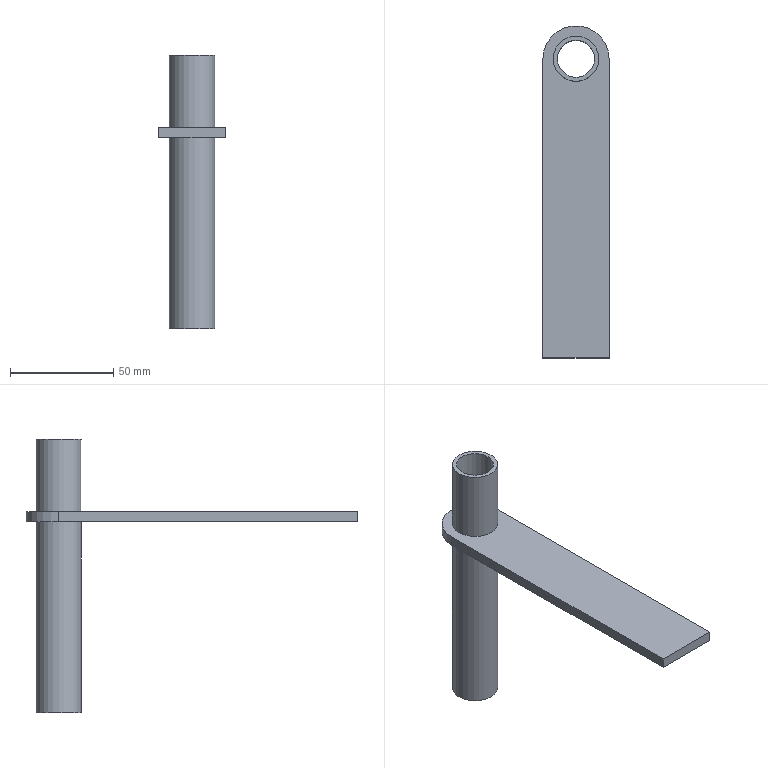Part | NX | features EXTRUDE 3, DATUM_CSYS 1, EXTRACT_DATUM_PLANE 1, SKETCH 1, UNITE 1 | 1 solid | 11 faces | box 32 x 161 x 132.5 mm | volume 39960 mm3 | plane 7 | cylinder 4 | commonest cylinder face diameters 22 x2 18 x1 32 x1
STEP:
#1=CARTESIAN_POINT('',(-16.,35.,-467.5));
#2=VERTEX_POINT('',#1);
#3=CARTESIAN_POINT('',(-16.,180.,-467.5));
#4=VERTEX_POINT('',#3);
#5=CARTESIAN_POINT('',(-16.,35.,-467.5));
#6=DIRECTION('',(0.,1.,0.));
#7=VECTOR('',#6,1000.);
#8=LINE('',#5,#7);
#9=EDGE_CURVE('',#2,#4,#8,.T.);
#10=ORIENTED_EDGE('',*,*,#9,.T.);
#11=CARTESIAN_POINT('',(-16.,180.,-472.5));
#12=VERTEX_POINT('',#11);
#13=CARTESIAN_POINT('',(-16.,180.,-472.5));
#14=DIRECTION('',(0.,0.,1.));
#15=VECTOR('',#14,1000.);
#16=LINE('',#13,#15);
#17=EDGE_CURVE('',#12,#4,#16,.T.);
#18=ORIENTED_EDGE('',*,*,#17,.F.);
#19=CARTESIAN_POINT('',(-16.,35.,-472.5));
#20=VERTEX_POINT('',#19);
#21=CARTESIAN_POINT('',(-16.,35.,-472.5));
#22=DIRECTION('',(0.,1.,0.));
#23=VECTOR('',#22,1000.);
#24=LINE('',#21,#23);
#25=EDGE_CURVE('',#20,#12,#24,.T.);
#26=ORIENTED_EDGE('',*,*,#25,.F.);
#27=CARTESIAN_POINT('',(-16.,35.,-472.5));
#28=DIRECTION('',(0.,0.,1.));
#29=VECTOR('',#28,1000.);
#30=LINE('',#27,#29);
#31=EDGE_CURVE('',#20,#2,#30,.T.);
#32=ORIENTED_EDGE('',*,*,#31,.T.);
#33=EDGE_LOOP('',(#10,#18,#26,#32));
#34=FACE_BOUND('',#33,.T.);
#35=CARTESIAN_POINT('',(-16.,35.,-472.5));
#36=DIRECTION('',(1.,0.,0.));
#37=DIRECTION('',(0.,0.,-1.));
#38=AXIS2_PLACEMENT_3D('',#35,#36,#37);
#39=PLANE('',#38);
#40=ADVANCED_FACE('',(#34),#39,.F.);
#41=CARTESIAN_POINT('',(16.,180.,-467.5));
#42=VERTEX_POINT('',#41);
#43=CARTESIAN_POINT('',(0.,180.,-467.5));
#44=DIRECTION('',(0.,0.,-1.));
#45=DIRECTION('',(-1.,0.,0.));
#46=AXIS2_PLACEMENT_3D('',#43,#44,#45);
#47=CIRCLE('',#46,16.);
#48=EDGE_CURVE('',#4,#42,#47,.T.);
#49=ORIENTED_EDGE('',*,*,#48,.T.);
#50=CARTESIAN_POINT('',(16.,180.,-472.5));
#51=VERTEX_POINT('',#50);
#52=CARTESIAN_POINT('',(16.,180.,-472.5));
#53=DIRECTION('',(0.,0.,1.));
#54=VECTOR('',#53,1000.);
#55=LINE('',#52,#54);
#56=EDGE_CURVE('',#51,#42,#55,.T.);
#57=ORIENTED_EDGE('',*,*,#56,.F.);
#58=CARTESIAN_POINT('',(0.,180.,-472.5));
#59=DIRECTION('',(0.,0.,-1.));
#60=DIRECTION('',(-1.,0.,0.));
#61=AXIS2_PLACEMENT_3D('',#58,#59,#60);
#62=CIRCLE('',#61,16.);
#63=EDGE_CURVE('',#12,#51,#62,.T.);
#64=ORIENTED_EDGE('',*,*,#63,.F.);
#65=ORIENTED_EDGE('',*,*,#17,.T.);
#66=EDGE_LOOP('',(#49,#57,#64,#65));
#67=FACE_BOUND('',#66,.T.);
#68=CARTESIAN_POINT('',(0.,180.,-472.5));
#69=DIRECTION('',(0.,0.,1.));
#70=DIRECTION('',(1.,0.,0.));
#71=AXIS2_PLACEMENT_3D('',#68,#69,#70);
#72=CYLINDRICAL_SURFACE('',#71,16.);
#73=ADVANCED_FACE('',(#67),#72,.T.);
#74=CARTESIAN_POINT('',(16.,35.,-467.5));
#75=VERTEX_POINT('',#74);
#76=CARTESIAN_POINT('',(16.,180.,-467.5));
#77=DIRECTION('',(0.,-1.,0.));
#78=VECTOR('',#77,1000.);
#79=LINE('',#76,#78);
#80=EDGE_CURVE('',#42,#75,#79,.T.);
#81=ORIENTED_EDGE('',*,*,#80,.T.);
#82=CARTESIAN_POINT('',(16.,35.,-472.5));
#83=VERTEX_POINT('',#82);
#84=CARTESIAN_POINT('',(16.,35.,-472.5));
#85=DIRECTION('',(0.,0.,1.));
#86=VECTOR('',#85,1000.);
#87=LINE('',#84,#86);
#88=EDGE_CURVE('',#83,#75,#87,.T.);
#89=ORIENTED_EDGE('',*,*,#88,.F.);
#90=CARTESIAN_POINT('',(16.,180.,-472.5));
#91=DIRECTION('',(0.,-1.,0.));
#92=VECTOR('',#91,1000.);
#93=LINE('',#90,#92);
#94=EDGE_CURVE('',#51,#83,#93,.T.);
#95=ORIENTED_EDGE('',*,*,#94,.F.);
#96=ORIENTED_EDGE('',*,*,#56,.T.);
#97=EDGE_LOOP('',(#81,#89,#95,#96));
#98=FACE_BOUND('',#97,.T.);
#99=CARTESIAN_POINT('',(16.,180.,-472.5));
#100=DIRECTION('',(-1.,0.,0.));
#101=DIRECTION('',(0.,0.,1.));
#102=AXIS2_PLACEMENT_3D('',#99,#100,#101);
#103=PLANE('',#102);
#104=ADVANCED_FACE('',(#98),#103,.F.);
#105=CARTESIAN_POINT('',(16.,35.,-467.5));
#106=DIRECTION('',(-1.,0.,0.));
#107=VECTOR('',#106,1000.);
#108=LINE('',#105,#107);
#109=EDGE_CURVE('',#75,#2,#108,.T.);
#110=ORIENTED_EDGE('',*,*,#109,.T.);
#111=ORIENTED_EDGE('',*,*,#31,.F.);
#112=CARTESIAN_POINT('',(16.,35.,-472.5));
#113=DIRECTION('',(-1.,0.,0.));
#114=VECTOR('',#113,1000.);
#115=LINE('',#112,#114);
#116=EDGE_CURVE('',#83,#20,#115,.T.);
#117=ORIENTED_EDGE('',*,*,#116,.F.);
#118=ORIENTED_EDGE('',*,*,#88,.T.);
#119=EDGE_LOOP('',(#110,#111,#117,#118));
#120=FACE_BOUND('',#119,.T.);
#121=CARTESIAN_POINT('',(16.,35.,-472.5));
#122=DIRECTION('',(0.,1.,0.));
#123=DIRECTION('',(0.,0.,1.));
#124=AXIS2_PLACEMENT_3D('',#121,#122,#123);
#125=PLANE('',#124);
#126=ADVANCED_FACE('',(#120),#125,.F.);
#127=CARTESIAN_POINT('',(-11.,180.,-472.5));
#128=VERTEX_POINT('',#127);
#129=CARTESIAN_POINT('',(0.,180.,-472.5));
#130=DIRECTION('',(0.,0.,-1.));
#131=DIRECTION('',(-1.,0.,0.));
#132=AXIS2_PLACEMENT_3D('',#129,#130,#131);
#133=CIRCLE('',#132,11.);
#134=EDGE_CURVE('',#128,#128,#133,.T.);
#135=ORIENTED_EDGE('',*,*,#134,.F.);
#136=EDGE_LOOP('',(#135));
#137=FACE_BOUND('',#136,.T.);
#138=ORIENTED_EDGE('',*,*,#25,.T.);
#139=ORIENTED_EDGE('',*,*,#63,.T.);
#140=ORIENTED_EDGE('',*,*,#94,.T.);
#141=ORIENTED_EDGE('',*,*,#116,.T.);
#142=EDGE_LOOP('',(#138,#139,#140,#141));
#143=FACE_BOUND('',#142,.T.);
#144=CARTESIAN_POINT('',(0.,180.,-472.5));
#145=DIRECTION('',(0.,0.,-1.));
#146=DIRECTION('',(-1.,0.,0.));
#147=AXIS2_PLACEMENT_3D('',#144,#145,#146);
#148=PLANE('',#147);
#149=ADVANCED_FACE('',(#137,#143),#148,.T.);
#150=CARTESIAN_POINT('',(-11.,180.,-467.5));
#151=VERTEX_POINT('',#150);
#152=CARTESIAN_POINT('',(0.,180.,-467.5));
#153=DIRECTION('',(0.,0.,-1.));
#154=DIRECTION('',(-1.,0.,0.));
#155=AXIS2_PLACEMENT_3D('',#152,#153,#154);
#156=CIRCLE('',#155,11.);
#157=EDGE_CURVE('',#151,#151,#156,.T.);
#158=ORIENTED_EDGE('',*,*,#157,.T.);
#159=EDGE_LOOP('',(#158));
#160=FACE_BOUND('',#159,.T.);
#161=ORIENTED_EDGE('',*,*,#9,.F.);
#162=ORIENTED_EDGE('',*,*,#109,.F.);
#163=ORIENTED_EDGE('',*,*,#80,.F.);
#164=ORIENTED_EDGE('',*,*,#48,.F.);
#165=EDGE_LOOP('',(#161,#162,#163,#164));
#166=FACE_BOUND('',#165,.T.);
#167=CARTESIAN_POINT('',(0.,180.,-467.5));
#168=DIRECTION('',(0.,0.,-1.));
#169=DIRECTION('',(-1.,0.,0.));
#170=AXIS2_PLACEMENT_3D('',#167,#168,#169);
#171=PLANE('',#170);
#172=ADVANCED_FACE('',(#160,#166),#171,.F.);
#173=CARTESIAN_POINT('',(11.,180.,-432.5));
#174=VERTEX_POINT('',#173);
#175=CARTESIAN_POINT('',(0.,180.,-432.5));
#176=DIRECTION('',(0.,0.,-1.));
#177=DIRECTION('',(1.,0.,0.));
#178=AXIS2_PLACEMENT_3D('',#175,#176,#177);
#179=CIRCLE('',#178,11.);
#180=EDGE_CURVE('',#174,#174,#179,.T.);
#181=ORIENTED_EDGE('',*,*,#180,.F.);
#182=EDGE_LOOP('',(#181));
#183=FACE_BOUND('',#182,.T.);
#184=CARTESIAN_POINT('',(9.,180.,-432.5));
#185=VERTEX_POINT('',#184);
#186=CARTESIAN_POINT('',(0.,180.,-432.5));
#187=DIRECTION('',(0.,0.,1.));
#188=DIRECTION('',(1.,0.,0.));
#189=AXIS2_PLACEMENT_3D('',#186,#187,#188);
#190=CIRCLE('',#189,9.);
#191=EDGE_CURVE('',#185,#185,#190,.T.);
#192=ORIENTED_EDGE('',*,*,#191,.F.);
#193=EDGE_LOOP('',(#192));
#194=FACE_BOUND('',#193,.T.);
#195=CARTESIAN_POINT('',(0.,180.,-432.5));
#196=DIRECTION('',(0.,0.,-1.));
#197=DIRECTION('',(-1.,0.,0.));
#198=AXIS2_PLACEMENT_3D('',#195,#196,#197);
#199=PLANE('',#198);
#200=ADVANCED_FACE('',(#183,#194),#199,.F.);
#201=ORIENTED_EDGE('',*,*,#180,.T.);
#202=EDGE_LOOP('',(#201));
#203=FACE_BOUND('',#202,.T.);
#204=ORIENTED_EDGE('',*,*,#157,.F.);
#205=EDGE_LOOP('',(#204));
#206=FACE_BOUND('',#205,.T.);
#207=CARTESIAN_POINT('',(0.,180.,-432.5));
#208=DIRECTION('',(0.,0.,-1.));
#209=DIRECTION('',(-1.,0.,0.));
#210=AXIS2_PLACEMENT_3D('',#207,#208,#209);
#211=CYLINDRICAL_SURFACE('',#210,11.);
#212=ADVANCED_FACE('',(#203,#206),#211,.T.);
#213=ORIENTED_EDGE('',*,*,#134,.T.);
#214=EDGE_LOOP('',(#213));
#215=FACE_BOUND('',#214,.T.);
#216=CARTESIAN_POINT('',(-11.,180.,-565.));
#217=VERTEX_POINT('',#216);
#218=CARTESIAN_POINT('',(0.,180.,-565.));
#219=DIRECTION('',(0.,0.,-1.));
#220=DIRECTION('',(-1.,0.,0.));
#221=AXIS2_PLACEMENT_3D('',#218,#219,#220);
#222=CIRCLE('',#221,11.);
#223=EDGE_CURVE('',#217,#217,#222,.T.);
#224=ORIENTED_EDGE('',*,*,#223,.F.);
#225=EDGE_LOOP('',(#224));
#226=FACE_BOUND('',#225,.T.);
#227=CARTESIAN_POINT('',(0.,180.,-432.5));
#228=DIRECTION('',(0.,0.,-1.));
#229=DIRECTION('',(-1.,0.,0.));
#230=AXIS2_PLACEMENT_3D('',#227,#228,#229);
#231=CYLINDRICAL_SURFACE('',#230,11.);
#232=ADVANCED_FACE('',(#215,#226),#231,.T.);
#233=ORIENTED_EDGE('',*,*,#223,.T.);
#234=EDGE_LOOP('',(#233));
#235=FACE_BOUND('',#234,.T.);
#236=CARTESIAN_POINT('',(-9.,180.,-565.));
#237=VERTEX_POINT('',#236);
#238=CARTESIAN_POINT('',(0.,180.,-565.));
#239=DIRECTION('',(0.,0.,1.));
#240=DIRECTION('',(-1.,0.,0.));
#241=AXIS2_PLACEMENT_3D('',#238,#239,#240);
#242=CIRCLE('',#241,9.);
#243=EDGE_CURVE('',#237,#237,#242,.T.);
#244=ORIENTED_EDGE('',*,*,#243,.T.);
#245=EDGE_LOOP('',(#244));
#246=FACE_BOUND('',#245,.T.);
#247=CARTESIAN_POINT('',(0.,180.,-565.));
#248=DIRECTION('',(0.,0.,-1.));
#249=DIRECTION('',(-1.,0.,0.));
#250=AXIS2_PLACEMENT_3D('',#247,#248,#249);
#251=PLANE('',#250);
#252=ADVANCED_FACE('',(#235,#246),#251,.T.);
#253=ORIENTED_EDGE('',*,*,#191,.T.);
#254=EDGE_LOOP('',(#253));
#255=FACE_BOUND('',#254,.T.);
#256=ORIENTED_EDGE('',*,*,#243,.F.);
#257=EDGE_LOOP('',(#256));
#258=FACE_BOUND('',#257,.T.);
#259=CARTESIAN_POINT('',(0.,180.,-432.5));
#260=DIRECTION('',(0.,0.,-1.));
#261=DIRECTION('',(-1.,0.,0.));
#262=AXIS2_PLACEMENT_3D('',#259,#260,#261);
#263=CYLINDRICAL_SURFACE('',#262,9.);
#264=ADVANCED_FACE('',(#255,#258),#263,.F.);
#265=CLOSED_SHELL('',(#40,#73,#104,#126,#149,#172,#200,#212,#232,#252,#264));
#266=MANIFOLD_SOLID_BREP('',#265);
#267=(LENGTH_UNIT()NAMED_UNIT(*)SI_UNIT(.MILLI.,.METRE.));
#268=UNCERTAINTY_MEASURE_WITH_UNIT(LENGTH_MEASURE(0.00001),#267,'','');
#269=(NAMED_UNIT(*)PLANE_ANGLE_UNIT()SI_UNIT($,.RADIAN.));
#270=(NAMED_UNIT(*)SI_UNIT($,.STERADIAN.)SOLID_ANGLE_UNIT());
#271=(GEOMETRIC_REPRESENTATION_CONTEXT(3)GLOBAL_UNCERTAINTY_ASSIGNED_CONTEXT((#268))GLOBAL_UNIT_ASSIGNED_CONTEXT((#267,#269,#270))REPRESENTATION_CONTEXT('',''));
#272=ADVANCED_BREP_SHAPE_REPRESENTATION('',(#266),#271);